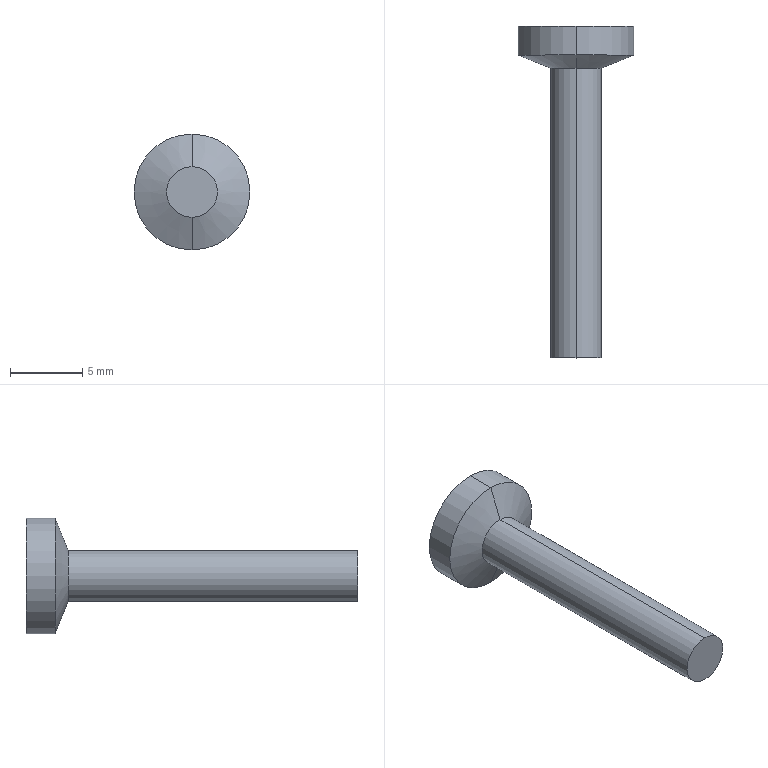Part | SolidWorks | features Revolution 1 | 1 solid | 8 faces | box 8 x 22.9 x 8 mm | volume 317.503 mm3 | cylinder 4 | cone 2 | plane 2 | commonest cylinder face diameters 3.5 x2 8 x2
STEP:
#1=CARTESIAN_POINT('',(0.,7.1,1.75));
#2=VERTEX_POINT('',#1);
#3=CARTESIAN_POINT('',(0.,7.1,-1.75));
#4=VERTEX_POINT('',#3);
#5=CARTESIAN_POINT('',(0.,7.1,0.));
#6=DIRECTION('',(0.,1.,0.));
#7=DIRECTION('',(0.,0.,1.));
#8=AXIS2_PLACEMENT_3D('',#5,#6,#7);
#9=CIRCLE('',#8,1.75);
#10=EDGE_CURVE('',#2,#4,#9,.T.);
#11=ORIENTED_EDGE('',*,*,#10,.T.);
#12=CARTESIAN_POINT('',(0.,27.1,-1.75));
#13=VERTEX_POINT('',#12);
#14=CARTESIAN_POINT('',(0.,30.,-1.75));
#15=DIRECTION('',(0.,1.,0.));
#16=VECTOR('',#15,1000.);
#17=LINE('',#14,#16);
#18=EDGE_CURVE('',#4,#13,#17,.T.);
#19=ORIENTED_EDGE('',*,*,#18,.T.);
#20=CARTESIAN_POINT('',(0.,27.1,1.75));
#21=VERTEX_POINT('',#20);
#22=CARTESIAN_POINT('',(0.,27.1,0.));
#23=DIRECTION('',(0.,1.,0.));
#24=DIRECTION('',(0.,0.,1.));
#25=AXIS2_PLACEMENT_3D('',#22,#23,#24);
#26=CIRCLE('',#25,1.75);
#27=EDGE_CURVE('',#21,#13,#26,.T.);
#28=ORIENTED_EDGE('',*,*,#27,.F.);
#29=CARTESIAN_POINT('',(0.,30.,1.75));
#30=DIRECTION('',(0.,1.,0.));
#31=VECTOR('',#30,1000.);
#32=LINE('',#29,#31);
#33=EDGE_CURVE('',#2,#21,#32,.T.);
#34=ORIENTED_EDGE('',*,*,#33,.F.);
#35=EDGE_LOOP('',(#11,#19,#28,#34));
#36=FACE_OUTER_BOUND('',#35,.T.);
#37=CARTESIAN_POINT('',(0.,30.,0.));
#38=DIRECTION('',(0.,1.,0.));
#39=DIRECTION('',(0.,0.,1.));
#40=AXIS2_PLACEMENT_3D('',#37,#38,#39);
#41=CYLINDRICAL_SURFACE('',#40,1.75);
#42=ADVANCED_FACE('',(#36),#41,.T.);
#43=CARTESIAN_POINT('',(0.,28.,4.));
#44=VERTEX_POINT('',#43);
#45=CARTESIAN_POINT('',(0.,28.,-4.));
#46=VERTEX_POINT('',#45);
#47=CARTESIAN_POINT('',(0.,28.,0.));
#48=DIRECTION('',(0.,1.,0.));
#49=DIRECTION('',(0.,0.,1.));
#50=AXIS2_PLACEMENT_3D('',#47,#48,#49);
#51=CIRCLE('',#50,4.);
#52=EDGE_CURVE('',#44,#46,#51,.T.);
#53=ORIENTED_EDGE('',*,*,#52,.T.);
#54=CARTESIAN_POINT('',(0.,30.,-4.));
#55=VERTEX_POINT('',#54);
#56=CARTESIAN_POINT('',(0.,30.,-4.));
#57=DIRECTION('',(0.,1.,0.));
#58=VECTOR('',#57,1000.);
#59=LINE('',#56,#58);
#60=EDGE_CURVE('',#46,#55,#59,.T.);
#61=ORIENTED_EDGE('',*,*,#60,.T.);
#62=CARTESIAN_POINT('',(0.,30.,4.));
#63=VERTEX_POINT('',#62);
#64=CARTESIAN_POINT('',(0.,30.,0.));
#65=DIRECTION('',(0.,1.,0.));
#66=DIRECTION('',(0.,0.,1.));
#67=AXIS2_PLACEMENT_3D('',#64,#65,#66);
#68=CIRCLE('',#67,4.);
#69=EDGE_CURVE('',#63,#55,#68,.T.);
#70=ORIENTED_EDGE('',*,*,#69,.F.);
#71=CARTESIAN_POINT('',(0.,30.,4.));
#72=DIRECTION('',(0.,1.,0.));
#73=VECTOR('',#72,1000.);
#74=LINE('',#71,#73);
#75=EDGE_CURVE('',#44,#63,#74,.T.);
#76=ORIENTED_EDGE('',*,*,#75,.F.);
#77=EDGE_LOOP('',(#53,#61,#70,#76));
#78=FACE_OUTER_BOUND('',#77,.T.);
#79=CARTESIAN_POINT('',(0.,30.,0.));
#80=DIRECTION('',(0.,1.,0.));
#81=DIRECTION('',(0.,0.,1.));
#82=AXIS2_PLACEMENT_3D('',#79,#80,#81);
#83=CYLINDRICAL_SURFACE('',#82,4.);
#84=ADVANCED_FACE('',(#78),#83,.T.);
#85=ORIENTED_EDGE('',*,*,#27,.T.);
#86=CARTESIAN_POINT('',(0.,27.1,-1.75));
#87=DIRECTION('',(0.,0.3712,-0.9285));
#88=VECTOR('',#87,1000.);
#89=LINE('',#86,#88);
#90=EDGE_CURVE('',#13,#46,#89,.T.);
#91=ORIENTED_EDGE('',*,*,#90,.T.);
#92=ORIENTED_EDGE('',*,*,#52,.F.);
#93=CARTESIAN_POINT('',(0.,27.1,1.75));
#94=DIRECTION('',(0.,0.3712,0.9285));
#95=VECTOR('',#94,1000.);
#96=LINE('',#93,#95);
#97=EDGE_CURVE('',#21,#44,#96,.T.);
#98=ORIENTED_EDGE('',*,*,#97,.F.);
#99=EDGE_LOOP('',(#85,#91,#92,#98));
#100=FACE_OUTER_BOUND('',#99,.T.);
#101=CARTESIAN_POINT('',(0.,27.1,0.));
#102=DIRECTION('',(0.,1.,0.));
#103=DIRECTION('',(0.,0.,1.));
#104=AXIS2_PLACEMENT_3D('',#101,#102,#103);
#105=CONICAL_SURFACE('',#104,1.75,1.19);
#106=ADVANCED_FACE('',(#100),#105,.T.);
#107=ORIENTED_EDGE('',*,*,#90,.F.);
#108=CARTESIAN_POINT('',(0.,27.1,0.));
#109=DIRECTION('',(0.,1.,0.));
#110=DIRECTION('',(0.,0.,1.));
#111=AXIS2_PLACEMENT_3D('',#108,#109,#110);
#112=CIRCLE('',#111,1.75);
#113=EDGE_CURVE('',#13,#21,#112,.T.);
#114=ORIENTED_EDGE('',*,*,#113,.T.);
#115=ORIENTED_EDGE('',*,*,#97,.T.);
#116=CARTESIAN_POINT('',(0.,28.,0.));
#117=DIRECTION('',(0.,1.,0.));
#118=DIRECTION('',(0.,0.,1.));
#119=AXIS2_PLACEMENT_3D('',#116,#117,#118);
#120=CIRCLE('',#119,4.);
#121=EDGE_CURVE('',#46,#44,#120,.T.);
#122=ORIENTED_EDGE('',*,*,#121,.F.);
#123=EDGE_LOOP('',(#107,#114,#115,#122));
#124=FACE_OUTER_BOUND('',#123,.T.);
#125=CARTESIAN_POINT('',(0.,27.1,0.));
#126=DIRECTION('',(0.,1.,0.));
#127=DIRECTION('',(0.,0.,1.));
#128=AXIS2_PLACEMENT_3D('',#125,#126,#127);
#129=CONICAL_SURFACE('',#128,1.75,1.19);
#130=ADVANCED_FACE('',(#124),#129,.T.);
#131=ORIENTED_EDGE('',*,*,#60,.F.);
#132=ORIENTED_EDGE('',*,*,#121,.T.);
#133=ORIENTED_EDGE('',*,*,#75,.T.);
#134=CARTESIAN_POINT('',(0.,30.,0.));
#135=DIRECTION('',(0.,1.,0.));
#136=DIRECTION('',(0.,0.,1.));
#137=AXIS2_PLACEMENT_3D('',#134,#135,#136);
#138=CIRCLE('',#137,4.);
#139=EDGE_CURVE('',#55,#63,#138,.T.);
#140=ORIENTED_EDGE('',*,*,#139,.F.);
#141=EDGE_LOOP('',(#131,#132,#133,#140));
#142=FACE_OUTER_BOUND('',#141,.T.);
#143=CARTESIAN_POINT('',(0.,30.,0.));
#144=DIRECTION('',(0.,1.,0.));
#145=DIRECTION('',(0.,0.,1.));
#146=AXIS2_PLACEMENT_3D('',#143,#144,#145);
#147=CYLINDRICAL_SURFACE('',#146,4.);
#148=ADVANCED_FACE('',(#142),#147,.T.);
#149=ORIENTED_EDGE('',*,*,#69,.T.);
#150=ORIENTED_EDGE('',*,*,#139,.T.);
#151=EDGE_LOOP('',(#149,#150));
#152=FACE_OUTER_BOUND('',#151,.T.);
#153=CARTESIAN_POINT('',(0.,30.,0.));
#154=DIRECTION('',(0.,-1.,0.));
#155=DIRECTION('',(0.,0.,-1.));
#156=AXIS2_PLACEMENT_3D('',#153,#154,#155);
#157=PLANE('',#156);
#158=ADVANCED_FACE('',(#152),#157,.F.);
#159=ORIENTED_EDGE('',*,*,#10,.F.);
#160=CARTESIAN_POINT('',(0.,7.1,0.));
#161=DIRECTION('',(0.,1.,0.));
#162=DIRECTION('',(0.,0.,1.));
#163=AXIS2_PLACEMENT_3D('',#160,#161,#162);
#164=CIRCLE('',#163,1.75);
#165=EDGE_CURVE('',#4,#2,#164,.T.);
#166=ORIENTED_EDGE('',*,*,#165,.F.);
#167=EDGE_LOOP('',(#159,#166));
#168=FACE_OUTER_BOUND('',#167,.T.);
#169=CARTESIAN_POINT('',(1.75,7.1,0.));
#170=DIRECTION('',(0.,1.,0.));
#171=DIRECTION('',(0.,0.,1.));
#172=AXIS2_PLACEMENT_3D('',#169,#170,#171);
#173=PLANE('',#172);
#174=ADVANCED_FACE('',(#168),#173,.F.);
#175=ORIENTED_EDGE('',*,*,#18,.F.);
#176=ORIENTED_EDGE('',*,*,#165,.T.);
#177=ORIENTED_EDGE('',*,*,#33,.T.);
#178=ORIENTED_EDGE('',*,*,#113,.F.);
#179=EDGE_LOOP('',(#175,#176,#177,#178));
#180=FACE_OUTER_BOUND('',#179,.T.);
#181=CARTESIAN_POINT('',(0.,30.,0.));
#182=DIRECTION('',(0.,1.,0.));
#183=DIRECTION('',(0.,0.,1.));
#184=AXIS2_PLACEMENT_3D('',#181,#182,#183);
#185=CYLINDRICAL_SURFACE('',#184,1.75);
#186=ADVANCED_FACE('',(#180),#185,.T.);
#187=CLOSED_SHELL('',(#42,#84,#106,#130,#148,#158,#174,#186));
#188=MANIFOLD_SOLID_BREP('',#187);
#189=CARTESIAN_POINT('',(0.,0.,0.));
#190=DIRECTION('',(0.,0.,1.));
#191=DIRECTION('',(1.,0.,0.));
#192=AXIS2_PLACEMENT_3D('',#189,#190,#191);
#193=(LENGTH_UNIT()NAMED_UNIT(*)SI_UNIT(.MILLI.,.METRE.));
#194=UNCERTAINTY_MEASURE_WITH_UNIT(LENGTH_MEASURE(0.00001),#193,'','');
#195=(NAMED_UNIT(*)PLANE_ANGLE_UNIT()SI_UNIT($,.RADIAN.));
#196=(NAMED_UNIT(*)SI_UNIT($,.STERADIAN.)SOLID_ANGLE_UNIT());
#197=(GEOMETRIC_REPRESENTATION_CONTEXT(3)GLOBAL_UNCERTAINTY_ASSIGNED_CONTEXT((#194))GLOBAL_UNIT_ASSIGNED_CONTEXT((#193,#195,#196))REPRESENTATION_CONTEXT('',''));
#198=ADVANCED_BREP_SHAPE_REPRESENTATION('',(#188,#192),#197);